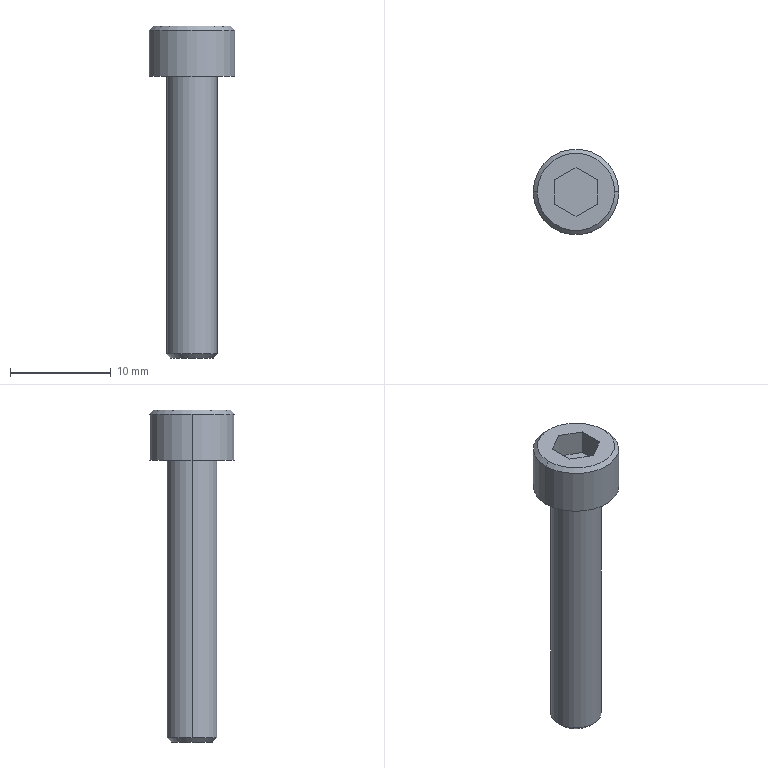Part | Creo | 1 solid | 18 faces | box 8.5 x 8.5 x 33 mm | volume 792.053 mm3 | plane 10 | cone 4 | cylinder 4 | commonest cylinder face diameters 5 x2 8.5 x2
STEP:
#1=CARTESIAN_POINT('',(-87.15,102.,40.099));
#2=VERTEX_POINT('',#1);
#3=CARTESIAN_POINT('',(-94.85,102.,40.099));
#4=VERTEX_POINT('',#3);
#5=CARTESIAN_POINT('',(-91.,102.,40.099));
#6=DIRECTION('',(0.,0.,1.));
#7=DIRECTION('',(1.,0.,0.));
#8=AXIS2_PLACEMENT_3D('',#5,#6,#7);
#9=CIRCLE('',#8,3.85);
#10=EDGE_CURVE('',#2,#4,#9,.T.);
#11=ORIENTED_EDGE('',*,*,#10,.F.);
#12=CARTESIAN_POINT('',(-91.,102.,40.099));
#13=DIRECTION('',(0.,0.,1.));
#14=DIRECTION('',(-1.,0.,0.));
#15=AXIS2_PLACEMENT_3D('',#12,#13,#14);
#16=CIRCLE('',#15,3.85);
#17=EDGE_CURVE('',#4,#2,#16,.T.);
#18=ORIENTED_EDGE('',*,*,#17,.F.);
#19=EDGE_LOOP('',(#11,#18));
#20=FACE_OUTER_BOUND('',#19,.F.);
#21=CARTESIAN_POINT('',(-93.1,100.788,40.099));
#22=VERTEX_POINT('',#21);
#23=CARTESIAN_POINT('',(-93.1,103.212,40.099));
#24=VERTEX_POINT('',#23);
#25=CARTESIAN_POINT('',(-93.1,100.788,40.099));
#26=DIRECTION('',(0.,1.,0.));
#27=VECTOR('',#26,2.425);
#28=LINE('',#25,#27);
#29=EDGE_CURVE('',#22,#24,#28,.T.);
#30=ORIENTED_EDGE('',*,*,#29,.F.);
#31=CARTESIAN_POINT('',(-91.,99.575,40.099));
#32=VERTEX_POINT('',#31);
#33=CARTESIAN_POINT('',(-91.,99.575,40.099));
#34=DIRECTION('',(-0.866,0.5,0.));
#35=VECTOR('',#34,2.425);
#36=LINE('',#33,#35);
#37=EDGE_CURVE('',#32,#22,#36,.T.);
#38=ORIENTED_EDGE('',*,*,#37,.F.);
#39=CARTESIAN_POINT('',(-88.9,100.788,40.099));
#40=VERTEX_POINT('',#39);
#41=CARTESIAN_POINT('',(-88.9,100.788,40.099));
#42=DIRECTION('',(-0.866,-0.5,0.));
#43=VECTOR('',#42,2.425);
#44=LINE('',#41,#43);
#45=EDGE_CURVE('',#40,#32,#44,.T.);
#46=ORIENTED_EDGE('',*,*,#45,.F.);
#47=CARTESIAN_POINT('',(-88.9,103.212,40.099));
#48=VERTEX_POINT('',#47);
#49=CARTESIAN_POINT('',(-88.9,103.212,40.099));
#50=DIRECTION('',(0.,-1.,0.));
#51=VECTOR('',#50,2.425);
#52=LINE('',#49,#51);
#53=EDGE_CURVE('',#48,#40,#52,.T.);
#54=ORIENTED_EDGE('',*,*,#53,.F.);
#55=CARTESIAN_POINT('',(-91.,104.425,40.099));
#56=VERTEX_POINT('',#55);
#57=CARTESIAN_POINT('',(-91.,104.425,40.099));
#58=DIRECTION('',(0.866,-0.5,0.));
#59=VECTOR('',#58,2.425);
#60=LINE('',#57,#59);
#61=EDGE_CURVE('',#56,#48,#60,.T.);
#62=ORIENTED_EDGE('',*,*,#61,.F.);
#63=CARTESIAN_POINT('',(-93.1,103.212,40.099));
#64=DIRECTION('',(0.866,0.5,0.));
#65=VECTOR('',#64,2.425);
#66=LINE('',#63,#65);
#67=EDGE_CURVE('',#24,#56,#66,.T.);
#68=ORIENTED_EDGE('',*,*,#67,.F.);
#69=EDGE_LOOP('',(#30,#38,#46,#54,#62,#68));
#70=FACE_BOUND('',#69,.F.);
#71=CARTESIAN_POINT('',(-91.,102.,40.099));
#72=DIRECTION('',(0.,0.,1.));
#73=DIRECTION('',(1.,0.,0.));
#74=AXIS2_PLACEMENT_3D('',#71,#72,#73);
#75=PLANE('',#74);
#76=ADVANCED_FACE('',(#20,#70),#75,.T.);
#77=ORIENTED_EDGE('',*,*,#10,.T.);
#78=CARTESIAN_POINT('',(-95.25,102.,39.699));
#79=VERTEX_POINT('',#78);
#80=CARTESIAN_POINT('',(-94.85,102.,40.099));
#81=DIRECTION('',(-0.7071,0.,-0.7071));
#82=VECTOR('',#81,0.5657);
#83=LINE('',#80,#82);
#84=EDGE_CURVE('',#4,#79,#83,.T.);
#85=ORIENTED_EDGE('',*,*,#84,.T.);
#86=CARTESIAN_POINT('',(-86.75,102.,39.699));
#87=VERTEX_POINT('',#86);
#88=CARTESIAN_POINT('',(-91.,102.,39.699));
#89=DIRECTION('',(0.,0.,1.));
#90=DIRECTION('',(1.,0.,0.));
#91=AXIS2_PLACEMENT_3D('',#88,#89,#90);
#92=CIRCLE('',#91,4.25);
#93=EDGE_CURVE('',#87,#79,#92,.T.);
#94=ORIENTED_EDGE('',*,*,#93,.F.);
#95=CARTESIAN_POINT('',(-87.15,102.,40.099));
#96=DIRECTION('',(0.7071,0.,-0.7071));
#97=VECTOR('',#96,0.5657);
#98=LINE('',#95,#97);
#99=EDGE_CURVE('',#2,#87,#98,.T.);
#100=ORIENTED_EDGE('',*,*,#99,.F.);
#101=EDGE_LOOP('',(#77,#85,#94,#100));
#102=FACE_OUTER_BOUND('',#101,.F.);
#103=CARTESIAN_POINT('',(-91.,102.,39.899));
#104=DIRECTION('',(0.,0.,-1.));
#105=DIRECTION('',(-1.,0.,0.));
#106=AXIS2_PLACEMENT_3D('',#103,#104,#105);
#107=CONICAL_SURFACE('',#106,4.05,45.);
#108=ADVANCED_FACE('',(#102),#107,.T.);
#109=ORIENTED_EDGE('',*,*,#17,.T.);
#110=ORIENTED_EDGE('',*,*,#99,.T.);
#111=CARTESIAN_POINT('',(-91.,102.,39.699));
#112=DIRECTION('',(0.,0.,1.));
#113=DIRECTION('',(-1.,0.,0.));
#114=AXIS2_PLACEMENT_3D('',#111,#112,#113);
#115=CIRCLE('',#114,4.25);
#116=EDGE_CURVE('',#79,#87,#115,.T.);
#117=ORIENTED_EDGE('',*,*,#116,.F.);
#118=ORIENTED_EDGE('',*,*,#84,.F.);
#119=EDGE_LOOP('',(#109,#110,#117,#118));
#120=FACE_OUTER_BOUND('',#119,.F.);
#121=CARTESIAN_POINT('',(-91.,102.,39.899));
#122=DIRECTION('',(0.,0.,-1.));
#123=DIRECTION('',(-1.,0.,0.));
#124=AXIS2_PLACEMENT_3D('',#121,#122,#123);
#125=CONICAL_SURFACE('',#124,4.05,45.);
#126=ADVANCED_FACE('',(#120),#125,.T.);
#127=ORIENTED_EDGE('',*,*,#116,.T.);
#128=CARTESIAN_POINT('',(-86.75,102.,35.099));
#129=VERTEX_POINT('',#128);
#130=CARTESIAN_POINT('',(-86.75,102.,35.099));
#131=DIRECTION('',(0.,0.,1.));
#132=VECTOR('',#131,4.6);
#133=LINE('',#130,#132);
#134=EDGE_CURVE('',#129,#87,#133,.T.);
#135=ORIENTED_EDGE('',*,*,#134,.F.);
#136=CARTESIAN_POINT('',(-95.25,102.,35.099));
#137=VERTEX_POINT('',#136);
#138=CARTESIAN_POINT('',(-91.,102.,35.099));
#139=DIRECTION('',(0.,0.,-1.));
#140=DIRECTION('',(1.,0.,0.));
#141=AXIS2_PLACEMENT_3D('',#138,#139,#140);
#142=CIRCLE('',#141,4.25);
#143=EDGE_CURVE('',#129,#137,#142,.T.);
#144=ORIENTED_EDGE('',*,*,#143,.T.);
#145=CARTESIAN_POINT('',(-95.25,102.,35.099));
#146=DIRECTION('',(0.,0.,1.));
#147=VECTOR('',#146,4.6);
#148=LINE('',#145,#147);
#149=EDGE_CURVE('',#137,#79,#148,.T.);
#150=ORIENTED_EDGE('',*,*,#149,.T.);
#151=EDGE_LOOP('',(#127,#135,#144,#150));
#152=FACE_OUTER_BOUND('',#151,.F.);
#153=CARTESIAN_POINT('',(-91.,102.,35.099));
#154=DIRECTION('',(0.,0.,1.));
#155=DIRECTION('',(1.,0.,0.));
#156=AXIS2_PLACEMENT_3D('',#153,#154,#155);
#157=CYLINDRICAL_SURFACE('',#156,4.25);
#158=ADVANCED_FACE('',(#152),#157,.T.);
#159=ORIENTED_EDGE('',*,*,#93,.T.);
#160=ORIENTED_EDGE('',*,*,#149,.F.);
#161=CARTESIAN_POINT('',(-91.,102.,35.099));
#162=DIRECTION('',(0.,0.,-1.));
#163=DIRECTION('',(-1.,0.,0.));
#164=AXIS2_PLACEMENT_3D('',#161,#162,#163);
#165=CIRCLE('',#164,4.25);
#166=EDGE_CURVE('',#137,#129,#165,.T.);
#167=ORIENTED_EDGE('',*,*,#166,.T.);
#168=ORIENTED_EDGE('',*,*,#134,.T.);
#169=EDGE_LOOP('',(#159,#160,#167,#168));
#170=FACE_OUTER_BOUND('',#169,.F.);
#171=CARTESIAN_POINT('',(-91.,102.,35.099));
#172=DIRECTION('',(0.,0.,1.));
#173=DIRECTION('',(1.,0.,0.));
#174=AXIS2_PLACEMENT_3D('',#171,#172,#173);
#175=CYLINDRICAL_SURFACE('',#174,4.25);
#176=ADVANCED_FACE('',(#170),#175,.T.);
#177=ORIENTED_EDGE('',*,*,#143,.F.);
#178=ORIENTED_EDGE('',*,*,#166,.F.);
#179=EDGE_LOOP('',(#177,#178));
#180=FACE_OUTER_BOUND('',#179,.F.);
#181=CARTESIAN_POINT('',(-93.5,102.,35.099));
#182=VERTEX_POINT('',#181);
#183=CARTESIAN_POINT('',(-88.5,102.,35.099));
#184=VERTEX_POINT('',#183);
#185=CARTESIAN_POINT('',(-91.,102.,35.099));
#186=DIRECTION('',(0.,0.,1.));
#187=DIRECTION('',(-1.,0.,0.));
#188=AXIS2_PLACEMENT_3D('',#185,#186,#187);
#189=CIRCLE('',#188,2.5);
#190=EDGE_CURVE('',#182,#184,#189,.T.);
#191=ORIENTED_EDGE('',*,*,#190,.F.);
#192=CARTESIAN_POINT('',(-91.,102.,35.099));
#193=DIRECTION('',(0.,0.,1.));
#194=DIRECTION('',(1.,0.,0.));
#195=AXIS2_PLACEMENT_3D('',#192,#193,#194);
#196=CIRCLE('',#195,2.5);
#197=EDGE_CURVE('',#184,#182,#196,.T.);
#198=ORIENTED_EDGE('',*,*,#197,.F.);
#199=EDGE_LOOP('',(#191,#198));
#200=FACE_BOUND('',#199,.F.);
#201=CARTESIAN_POINT('',(-91.,102.,35.099));
#202=DIRECTION('',(0.,0.,-1.));
#203=DIRECTION('',(-1.,0.,0.));
#204=AXIS2_PLACEMENT_3D('',#201,#202,#203);
#205=PLANE('',#204);
#206=ADVANCED_FACE('',(#180,#200),#205,.T.);
#207=CARTESIAN_POINT('',(-88.5,102.,7.499));
#208=VERTEX_POINT('',#207);
#209=CARTESIAN_POINT('',(-93.5,102.,7.499));
#210=VERTEX_POINT('',#209);
#211=CARTESIAN_POINT('',(-91.,102.,7.499));
#212=DIRECTION('',(0.,0.,-1.));
#213=DIRECTION('',(1.,0.,0.));
#214=AXIS2_PLACEMENT_3D('',#211,#212,#213);
#215=CIRCLE('',#214,2.5);
#216=EDGE_CURVE('',#208,#210,#215,.T.);
#217=ORIENTED_EDGE('',*,*,#216,.T.);
#218=CARTESIAN_POINT('',(-93.5,102.,35.099));
#219=DIRECTION('',(0.,0.,-1.));
#220=VECTOR('',#219,27.6);
#221=LINE('',#218,#220);
#222=EDGE_CURVE('',#182,#210,#221,.T.);
#223=ORIENTED_EDGE('',*,*,#222,.F.);
#224=ORIENTED_EDGE('',*,*,#190,.T.);
#225=CARTESIAN_POINT('',(-88.5,102.,35.099));
#226=DIRECTION('',(0.,0.,-1.));
#227=VECTOR('',#226,27.6);
#228=LINE('',#225,#227);
#229=EDGE_CURVE('',#184,#208,#228,.T.);
#230=ORIENTED_EDGE('',*,*,#229,.T.);
#231=EDGE_LOOP('',(#217,#223,#224,#230));
#232=FACE_OUTER_BOUND('',#231,.F.);
#233=CARTESIAN_POINT('',(-91.,102.,35.099));
#234=DIRECTION('',(0.,0.,-1.));
#235=DIRECTION('',(-1.,0.,0.));
#236=AXIS2_PLACEMENT_3D('',#233,#234,#235);
#237=CYLINDRICAL_SURFACE('',#236,2.5);
#238=ADVANCED_FACE('',(#232),#237,.T.);
#239=CARTESIAN_POINT('',(-88.9,102.,7.099));
#240=VERTEX_POINT('',#239);
#241=CARTESIAN_POINT('',(-93.1,102.,7.099));
#242=VERTEX_POINT('',#241);
#243=CARTESIAN_POINT('',(-91.,102.,7.099));
#244=DIRECTION('',(0.,0.,-1.));
#245=DIRECTION('',(1.,0.,0.));
#246=AXIS2_PLACEMENT_3D('',#243,#244,#245);
#247=CIRCLE('',#246,2.1);
#248=EDGE_CURVE('',#240,#242,#247,.T.);
#249=ORIENTED_EDGE('',*,*,#248,.T.);
#250=CARTESIAN_POINT('',(-93.1,102.,7.099));
#251=DIRECTION('',(-0.7071,0.,0.7071));
#252=VECTOR('',#251,0.5657);
#253=LINE('',#250,#252);
#254=EDGE_CURVE('',#242,#210,#253,.T.);
#255=ORIENTED_EDGE('',*,*,#254,.T.);
#256=ORIENTED_EDGE('',*,*,#216,.F.);
#257=CARTESIAN_POINT('',(-88.9,102.,7.099));
#258=DIRECTION('',(0.7071,0.,0.7071));
#259=VECTOR('',#258,0.5657);
#260=LINE('',#257,#259);
#261=EDGE_CURVE('',#240,#208,#260,.T.);
#262=ORIENTED_EDGE('',*,*,#261,.F.);
#263=EDGE_LOOP('',(#249,#255,#256,#262));
#264=FACE_OUTER_BOUND('',#263,.F.);
#265=CARTESIAN_POINT('',(-91.,102.,7.299));
#266=DIRECTION('',(0.,0.,1.));
#267=DIRECTION('',(1.,0.,0.));
#268=AXIS2_PLACEMENT_3D('',#265,#266,#267);
#269=CONICAL_SURFACE('',#268,2.3,45.);
#270=ADVANCED_FACE('',(#264),#269,.T.);
#271=CARTESIAN_POINT('',(-91.,102.,7.099));
#272=DIRECTION('',(0.,0.,-1.));
#273=DIRECTION('',(-1.,0.,0.));
#274=AXIS2_PLACEMENT_3D('',#271,#272,#273);
#275=CIRCLE('',#274,2.1);
#276=EDGE_CURVE('',#242,#240,#275,.T.);
#277=ORIENTED_EDGE('',*,*,#276,.F.);
#278=ORIENTED_EDGE('',*,*,#248,.F.);
#279=EDGE_LOOP('',(#277,#278));
#280=FACE_OUTER_BOUND('',#279,.F.);
#281=CARTESIAN_POINT('',(-91.,102.,7.099));
#282=DIRECTION('',(0.,0.,-1.));
#283=DIRECTION('',(-1.,0.,0.));
#284=AXIS2_PLACEMENT_3D('',#281,#282,#283);
#285=PLANE('',#284);
#286=ADVANCED_FACE('',(#280),#285,.T.);
#287=ORIENTED_EDGE('',*,*,#276,.T.);
#288=ORIENTED_EDGE('',*,*,#261,.T.);
#289=CARTESIAN_POINT('',(-91.,102.,7.499));
#290=DIRECTION('',(0.,0.,-1.));
#291=DIRECTION('',(-1.,0.,0.));
#292=AXIS2_PLACEMENT_3D('',#289,#290,#291);
#293=CIRCLE('',#292,2.5);
#294=EDGE_CURVE('',#210,#208,#293,.T.);
#295=ORIENTED_EDGE('',*,*,#294,.F.);
#296=ORIENTED_EDGE('',*,*,#254,.F.);
#297=EDGE_LOOP('',(#287,#288,#295,#296));
#298=FACE_OUTER_BOUND('',#297,.F.);
#299=CARTESIAN_POINT('',(-91.,102.,7.299));
#300=DIRECTION('',(0.,0.,1.));
#301=DIRECTION('',(1.,0.,0.));
#302=AXIS2_PLACEMENT_3D('',#299,#300,#301);
#303=CONICAL_SURFACE('',#302,2.3,45.);
#304=ADVANCED_FACE('',(#298),#303,.T.);
#305=ORIENTED_EDGE('',*,*,#294,.T.);
#306=ORIENTED_EDGE('',*,*,#229,.F.);
#307=ORIENTED_EDGE('',*,*,#197,.T.);
#308=ORIENTED_EDGE('',*,*,#222,.T.);
#309=EDGE_LOOP('',(#305,#306,#307,#308));
#310=FACE_OUTER_BOUND('',#309,.F.);
#311=CARTESIAN_POINT('',(-91.,102.,35.099));
#312=DIRECTION('',(0.,0.,-1.));
#313=DIRECTION('',(-1.,0.,0.));
#314=AXIS2_PLACEMENT_3D('',#311,#312,#313);
#315=CYLINDRICAL_SURFACE('',#314,2.5);
#316=ADVANCED_FACE('',(#310),#315,.T.);
#317=ORIENTED_EDGE('',*,*,#29,.T.);
#318=CARTESIAN_POINT('',(-93.1,103.212,37.599));
#319=VERTEX_POINT('',#318);
#320=CARTESIAN_POINT('',(-93.1,103.212,40.099));
#321=DIRECTION('',(0.,0.,-1.));
#322=VECTOR('',#321,2.5);
#323=LINE('',#320,#322);
#324=EDGE_CURVE('',#24,#319,#323,.T.);
#325=ORIENTED_EDGE('',*,*,#324,.T.);
#326=CARTESIAN_POINT('',(-93.1,100.788,37.599));
#327=VERTEX_POINT('',#326);
#328=CARTESIAN_POINT('',(-93.1,100.788,37.599));
#329=DIRECTION('',(0.,1.,0.));
#330=VECTOR('',#329,2.425);
#331=LINE('',#328,#330);
#332=EDGE_CURVE('',#327,#319,#331,.T.);
#333=ORIENTED_EDGE('',*,*,#332,.F.);
#334=CARTESIAN_POINT('',(-93.1,100.788,40.099));
#335=DIRECTION('',(0.,0.,-1.));
#336=VECTOR('',#335,2.5);
#337=LINE('',#334,#336);
#338=EDGE_CURVE('',#22,#327,#337,.T.);
#339=ORIENTED_EDGE('',*,*,#338,.F.);
#340=EDGE_LOOP('',(#317,#325,#333,#339));
#341=FACE_OUTER_BOUND('',#340,.F.);
#342=CARTESIAN_POINT('',(-93.1,102.,38.849));
#343=DIRECTION('',(-1.,0.,0.));
#344=DIRECTION('',(0.,0.,1.));
#345=AXIS2_PLACEMENT_3D('',#342,#343,#344);
#346=PLANE('',#345);
#347=ADVANCED_FACE('',(#341),#346,.F.);
#348=ORIENTED_EDGE('',*,*,#67,.T.);
#349=CARTESIAN_POINT('',(-91.,104.425,37.599));
#350=VERTEX_POINT('',#349);
#351=CARTESIAN_POINT('',(-91.,104.425,40.099));
#352=DIRECTION('',(0.,0.,-1.));
#353=VECTOR('',#352,2.5);
#354=LINE('',#351,#353);
#355=EDGE_CURVE('',#56,#350,#354,.T.);
#356=ORIENTED_EDGE('',*,*,#355,.T.);
#357=CARTESIAN_POINT('',(-91.,104.425,37.599));
#358=DIRECTION('',(-0.866,-0.5,0.));
#359=VECTOR('',#358,2.425);
#360=LINE('',#357,#359);
#361=EDGE_CURVE('',#350,#319,#360,.T.);
#362=ORIENTED_EDGE('',*,*,#361,.T.);
#363=ORIENTED_EDGE('',*,*,#324,.F.);
#364=EDGE_LOOP('',(#348,#356,#362,#363));
#365=FACE_OUTER_BOUND('',#364,.F.);
#366=CARTESIAN_POINT('',(-92.05,103.819,38.849));
#367=DIRECTION('',(-0.5,0.866,0.));
#368=DIRECTION('',(-0.866,-0.5,0.));
#369=AXIS2_PLACEMENT_3D('',#366,#367,#368);
#370=PLANE('',#369);
#371=ADVANCED_FACE('',(#365),#370,.F.);
#372=ORIENTED_EDGE('',*,*,#61,.T.);
#373=CARTESIAN_POINT('',(-88.9,103.212,37.599));
#374=VERTEX_POINT('',#373);
#375=CARTESIAN_POINT('',(-88.9,103.212,40.099));
#376=DIRECTION('',(0.,0.,-1.));
#377=VECTOR('',#376,2.5);
#378=LINE('',#375,#377);
#379=EDGE_CURVE('',#48,#374,#378,.T.);
#380=ORIENTED_EDGE('',*,*,#379,.T.);
#381=CARTESIAN_POINT('',(-88.9,103.212,37.599));
#382=DIRECTION('',(-0.866,0.5,0.));
#383=VECTOR('',#382,2.425);
#384=LINE('',#381,#383);
#385=EDGE_CURVE('',#374,#350,#384,.T.);
#386=ORIENTED_EDGE('',*,*,#385,.T.);
#387=ORIENTED_EDGE('',*,*,#355,.F.);
#388=EDGE_LOOP('',(#372,#380,#386,#387));
#389=FACE_OUTER_BOUND('',#388,.F.);
#390=CARTESIAN_POINT('',(-89.95,103.819,38.849));
#391=DIRECTION('',(0.5,0.866,0.));
#392=DIRECTION('',(-0.866,0.5,0.));
#393=AXIS2_PLACEMENT_3D('',#390,#391,#392);
#394=PLANE('',#393);
#395=ADVANCED_FACE('',(#389),#394,.F.);
#396=ORIENTED_EDGE('',*,*,#53,.T.);
#397=CARTESIAN_POINT('',(-88.9,100.788,37.599));
#398=VERTEX_POINT('',#397);
#399=CARTESIAN_POINT('',(-88.9,100.788,40.099));
#400=DIRECTION('',(0.,0.,-1.));
#401=VECTOR('',#400,2.5);
#402=LINE('',#399,#401);
#403=EDGE_CURVE('',#40,#398,#402,.T.);
#404=ORIENTED_EDGE('',*,*,#403,.T.);
#405=CARTESIAN_POINT('',(-88.9,103.212,37.599));
#406=DIRECTION('',(0.,-1.,0.));
#407=VECTOR('',#406,2.425);
#408=LINE('',#405,#407);
#409=EDGE_CURVE('',#374,#398,#408,.T.);
#410=ORIENTED_EDGE('',*,*,#409,.F.);
#411=ORIENTED_EDGE('',*,*,#379,.F.);
#412=EDGE_LOOP('',(#396,#404,#410,#411));
#413=FACE_OUTER_BOUND('',#412,.F.);
#414=CARTESIAN_POINT('',(-88.9,102.,38.849));
#415=DIRECTION('',(1.,0.,0.));
#416=DIRECTION('',(0.,0.,-1.));
#417=AXIS2_PLACEMENT_3D('',#414,#415,#416);
#418=PLANE('',#417);
#419=ADVANCED_FACE('',(#413),#418,.F.);
#420=ORIENTED_EDGE('',*,*,#45,.T.);
#421=CARTESIAN_POINT('',(-91.,99.575,37.599));
#422=VERTEX_POINT('',#421);
#423=CARTESIAN_POINT('',(-91.,99.575,40.099));
#424=DIRECTION('',(0.,0.,-1.));
#425=VECTOR('',#424,2.5);
#426=LINE('',#423,#425);
#427=EDGE_CURVE('',#32,#422,#426,.T.);
#428=ORIENTED_EDGE('',*,*,#427,.T.);
#429=CARTESIAN_POINT('',(-91.,99.575,37.599));
#430=DIRECTION('',(0.866,0.5,0.));
#431=VECTOR('',#430,2.425);
#432=LINE('',#429,#431);
#433=EDGE_CURVE('',#422,#398,#432,.T.);
#434=ORIENTED_EDGE('',*,*,#433,.T.);
#435=ORIENTED_EDGE('',*,*,#403,.F.);
#436=EDGE_LOOP('',(#420,#428,#434,#435));
#437=FACE_OUTER_BOUND('',#436,.F.);
#438=CARTESIAN_POINT('',(-89.95,100.181,38.849));
#439=DIRECTION('',(0.5,-0.866,0.));
#440=DIRECTION('',(0.866,0.5,0.));
#441=AXIS2_PLACEMENT_3D('',#438,#439,#440);
#442=PLANE('',#441);
#443=ADVANCED_FACE('',(#437),#442,.F.);
#444=ORIENTED_EDGE('',*,*,#37,.T.);
#445=ORIENTED_EDGE('',*,*,#338,.T.);
#446=CARTESIAN_POINT('',(-93.1,100.788,37.599));
#447=DIRECTION('',(0.866,-0.5,0.));
#448=VECTOR('',#447,2.425);
#449=LINE('',#446,#448);
#450=EDGE_CURVE('',#327,#422,#449,.T.);
#451=ORIENTED_EDGE('',*,*,#450,.T.);
#452=ORIENTED_EDGE('',*,*,#427,.F.);
#453=EDGE_LOOP('',(#444,#445,#451,#452));
#454=FACE_OUTER_BOUND('',#453,.F.);
#455=CARTESIAN_POINT('',(-92.05,100.181,38.849));
#456=DIRECTION('',(-0.5,-0.866,0.));
#457=DIRECTION('',(0.866,-0.5,0.));
#458=AXIS2_PLACEMENT_3D('',#455,#456,#457);
#459=PLANE('',#458);
#460=ADVANCED_FACE('',(#454),#459,.F.);
#461=ORIENTED_EDGE('',*,*,#433,.F.);
#462=ORIENTED_EDGE('',*,*,#450,.F.);
#463=ORIENTED_EDGE('',*,*,#332,.T.);
#464=ORIENTED_EDGE('',*,*,#361,.F.);
#465=ORIENTED_EDGE('',*,*,#385,.F.);
#466=ORIENTED_EDGE('',*,*,#409,.T.);
#467=EDGE_LOOP('',(#461,#462,#463,#464,#465,#466));
#468=FACE_OUTER_BOUND('',#467,.F.);
#469=CARTESIAN_POINT('',(-91.,102.,37.599));
#470=DIRECTION('',(0.,0.,-1.));
#471=DIRECTION('',(-1.,0.,0.));
#472=AXIS2_PLACEMENT_3D('',#469,#470,#471);
#473=PLANE('',#472);
#474=ADVANCED_FACE('',(#468),#473,.F.);
#475=CLOSED_SHELL('',(#76,#108,#126,#158,#176,#206,#238,#270,#286,#304,#316,#347,#371,#395,#419,#443,#460,#474));
#476=MANIFOLD_SOLID_BREP('',#475);
#477=(LENGTH_UNIT()NAMED_UNIT(*)SI_UNIT(.MILLI.,.METRE.));
#478=UNCERTAINTY_MEASURE_WITH_UNIT(LENGTH_MEASURE(0.003512),#477,'','');
#479=(NAMED_UNIT(*)PLANE_ANGLE_UNIT()SI_UNIT($,.RADIAN.));
#480=PLANE_ANGLE_MEASURE_WITH_UNIT(PLANE_ANGLE_MEASURE(0.01745),#479);
#481=(CONVERSION_BASED_UNIT('DEGREE',#480)NAMED_UNIT(*)PLANE_ANGLE_UNIT());
#482=(NAMED_UNIT(*)SI_UNIT($,.STERADIAN.)SOLID_ANGLE_UNIT());
#483=(GEOMETRIC_REPRESENTATION_CONTEXT(3)GLOBAL_UNCERTAINTY_ASSIGNED_CONTEXT((#478))GLOBAL_UNIT_ASSIGNED_CONTEXT((#477,#481,#482))REPRESENTATION_CONTEXT('',''));
#484=ADVANCED_BREP_SHAPE_REPRESENTATION('',(#476),#483);